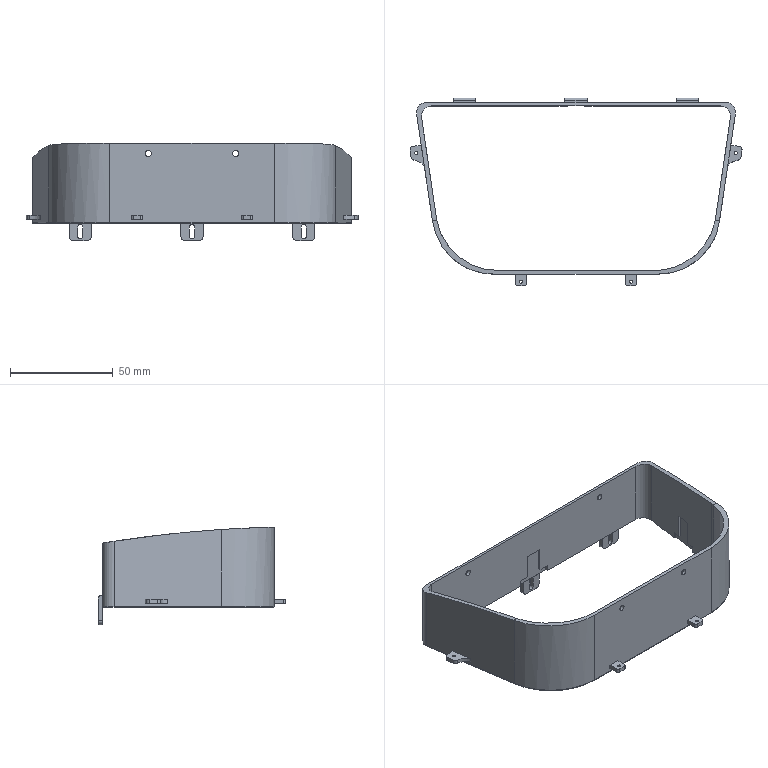Part | SolidWorks | features SavedExtBody 1 | 1 solid | 147 faces | box 161.389 x 91.111 x 47.426 mm | volume 30382 mm3 | plane 85 | cylinder 54 | spline 4 | torus 4 | commonest cylinder face diameters 3 x12 2.5 x9 1.5 x8 2 x7 4 x6 1 x4